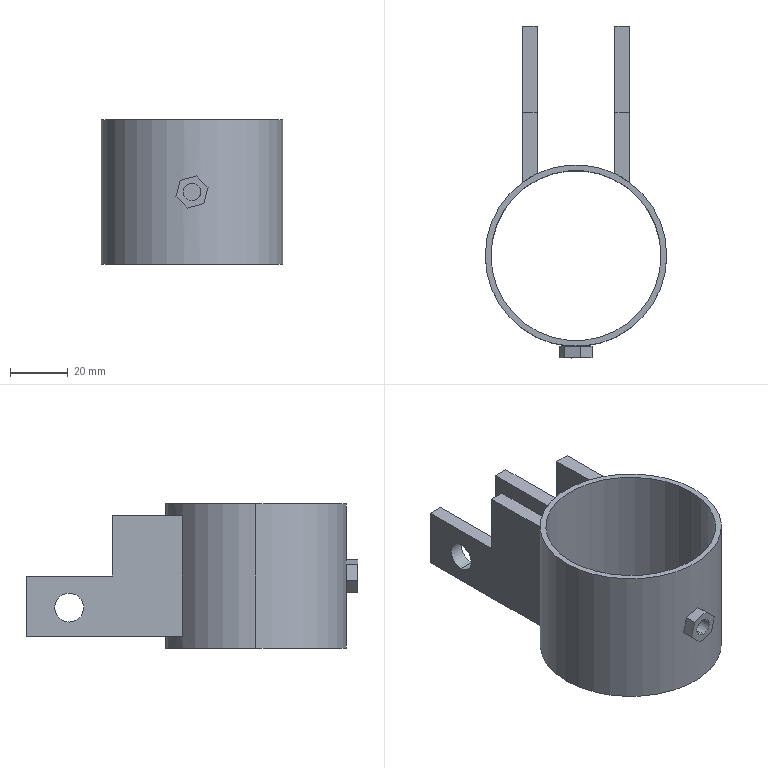Part | SolidWorks | features ICE 5, Extrusion 1 | 2 solids | 36 faces | box 63 x 115.25 x 50 mm | volume 34376 mm3 | plane 24 | cylinder 12 | commonest cylinder face diameters 6 x4 10 x4 59 x2 63 x2
STEP:
#1=CARTESIAN_POINT('',(0.,-31.5,22.));
#2=VERTEX_POINT('',#1);
#3=CARTESIAN_POINT('',(0.,-31.5,28.));
#4=VERTEX_POINT('',#3);
#5=CARTESIAN_POINT('',(0.,-31.5,22.));
#6=CARTESIAN_POINT('',(-0.1958,-31.5,22.));
#7=CARTESIAN_POINT('',(-0.3905,-31.498,22.019));
#8=CARTESIAN_POINT('',(-0.7776,-31.491,22.096));
#9=CARTESIAN_POINT('',(-0.967,-31.486,22.153));
#10=CARTESIAN_POINT('',(-1.328,-31.473,22.303));
#11=CARTESIAN_POINT('',(-1.502,-31.465,22.396));
#12=CARTESIAN_POINT('',(-1.83,-31.447,22.615));
#13=CARTESIAN_POINT('',(-1.981,-31.438,22.739));
#14=CARTESIAN_POINT('',(-2.258,-31.419,23.015));
#15=CARTESIAN_POINT('',(-2.385,-31.41,23.17));
#16=CARTESIAN_POINT('',(-2.603,-31.392,23.495));
#17=CARTESIAN_POINT('',(-2.695,-31.385,23.668));
#18=CARTESIAN_POINT('',(-2.846,-31.371,24.031));
#19=CARTESIAN_POINT('',(-2.904,-31.366,24.221));
#20=CARTESIAN_POINT('',(-2.98,-31.359,24.605));
#21=CARTESIAN_POINT('',(-3.,-31.357,24.8));
#22=CARTESIAN_POINT('',(-3.,-31.357,25.196));
#23=CARTESIAN_POINT('',(-2.981,-31.359,25.391));
#24=CARTESIAN_POINT('',(-2.905,-31.366,25.775));
#25=CARTESIAN_POINT('',(-2.847,-31.371,25.965));
#26=CARTESIAN_POINT('',(-2.697,-31.384,26.329));
#27=CARTESIAN_POINT('',(-2.605,-31.392,26.501));
#28=CARTESIAN_POINT('',(-2.388,-31.41,26.827));
#29=CARTESIAN_POINT('',(-2.261,-31.419,26.981));
#30=CARTESIAN_POINT('',(-1.985,-31.438,27.258));
#31=CARTESIAN_POINT('',(-1.834,-31.447,27.382));
#32=CARTESIAN_POINT('',(-1.506,-31.464,27.602));
#33=CARTESIAN_POINT('',(-1.332,-31.472,27.695));
#34=CARTESIAN_POINT('',(-0.7906,-31.492,27.92));
#35=CARTESIAN_POINT('',(-0.3966,-31.5,28.));
#36=CARTESIAN_POINT('',(0.,-31.5,28.));
#37=B_SPLINE_CURVE_WITH_KNOTS('',3,(#5,#6,#7,#8,#9,#10,#11,#12,#13,#14,#15,#16,#17,#18,#19,#20,#21,#22,#23,#24,#25,#26,#27,#28,#29,#30,#31,#32,#33,#34,#35,#36),.UNSPECIFIED.,.F.,.F.,(4,2,2,2,2,2,2,2,2,2,2,2,2,2,2,4),(0.009385,0.009971,0.01056,0.01114,0.01173,0.01232,0.0129,0.01349,0.01408,0.01466,0.01525,0.01584,0.01642,0.01701,0.01759,0.01877),.UNSPECIFIED.);
#38=EDGE_CURVE('',#2,#4,#37,.T.);
#39=ORIENTED_EDGE('',*,*,#38,.F.);
#40=CARTESIAN_POINT('',(0.,-29.5,22.));
#41=VERTEX_POINT('',#40);
#42=CARTESIAN_POINT('',(0.,-55.,22.));
#43=DIRECTION('',(0.,1.,0.));
#44=VECTOR('',#43,1000.);
#45=LINE('',#42,#44);
#46=EDGE_CURVE('',#2,#41,#45,.T.);
#47=ORIENTED_EDGE('',*,*,#46,.T.);
#48=CARTESIAN_POINT('',(0.,-29.5,28.));
#49=VERTEX_POINT('',#48);
#50=CARTESIAN_POINT('',(0.,-29.5,22.));
#51=CARTESIAN_POINT('',(-0.1958,-29.5,22.));
#52=CARTESIAN_POINT('',(-0.3905,-29.498,22.019));
#53=CARTESIAN_POINT('',(-0.7776,-29.49,22.096));
#54=CARTESIAN_POINT('',(-0.967,-29.485,22.153));
#55=CARTESIAN_POINT('',(-1.328,-29.471,22.303));
#56=CARTESIAN_POINT('',(-1.502,-29.462,22.396));
#57=CARTESIAN_POINT('',(-1.83,-29.444,22.615));
#58=CARTESIAN_POINT('',(-1.982,-29.434,22.739));
#59=CARTESIAN_POINT('',(-2.258,-29.414,23.015));
#60=CARTESIAN_POINT('',(-2.385,-29.404,23.17));
#61=CARTESIAN_POINT('',(-2.603,-29.385,23.495));
#62=CARTESIAN_POINT('',(-2.695,-29.377,23.668));
#63=CARTESIAN_POINT('',(-2.846,-29.363,24.031));
#64=CARTESIAN_POINT('',(-2.904,-29.357,24.221));
#65=CARTESIAN_POINT('',(-2.98,-29.349,24.605));
#66=CARTESIAN_POINT('',(-3.,-29.347,24.8));
#67=CARTESIAN_POINT('',(-3.,-29.347,25.196));
#68=CARTESIAN_POINT('',(-2.981,-29.349,25.391));
#69=CARTESIAN_POINT('',(-2.905,-29.357,25.775));
#70=CARTESIAN_POINT('',(-2.847,-29.362,25.965));
#71=CARTESIAN_POINT('',(-2.697,-29.377,26.329));
#72=CARTESIAN_POINT('',(-2.605,-29.385,26.501));
#73=CARTESIAN_POINT('',(-2.387,-29.403,26.827));
#74=CARTESIAN_POINT('',(-2.261,-29.414,26.981));
#75=CARTESIAN_POINT('',(-1.985,-29.433,27.258));
#76=CARTESIAN_POINT('',(-1.834,-29.443,27.382));
#77=CARTESIAN_POINT('',(-1.506,-29.462,27.602));
#78=CARTESIAN_POINT('',(-1.332,-29.47,27.695));
#79=CARTESIAN_POINT('',(-0.7907,-29.492,27.92));
#80=CARTESIAN_POINT('',(-0.3966,-29.5,28.));
#81=CARTESIAN_POINT('',(0.,-29.5,28.));
#82=B_SPLINE_CURVE_WITH_KNOTS('',3,(#50,#51,#52,#53,#54,#55,#56,#57,#58,#59,#60,#61,#62,#63,#64,#65,#66,#67,#68,#69,#70,#71,#72,#73,#74,#75,#76,#77,#78,#79,#80,#81),.UNSPECIFIED.,.F.,.F.,(4,2,2,2,2,2,2,2,2,2,2,2,2,2,2,4),(0.009385,0.009972,0.01056,0.01114,0.01173,0.01232,0.0129,0.01349,0.01408,0.01466,0.01525,0.01584,0.01642,0.01701,0.0176,0.01877),.UNSPECIFIED.);
#83=EDGE_CURVE('',#41,#49,#82,.T.);
#84=ORIENTED_EDGE('',*,*,#83,.T.);
#85=CARTESIAN_POINT('',(0.,-55.,28.));
#86=DIRECTION('',(0.,1.,0.));
#87=VECTOR('',#86,1000.);
#88=LINE('',#85,#87);
#89=EDGE_CURVE('',#4,#49,#88,.T.);
#90=ORIENTED_EDGE('',*,*,#89,.F.);
#91=EDGE_LOOP('',(#39,#47,#84,#90));
#92=FACE_OUTER_BOUND('',#91,.T.);
#93=CARTESIAN_POINT('',(0.,-55.,25.));
#94=DIRECTION('',(0.,1.,0.));
#95=DIRECTION('',(0.,0.,1.));
#96=AXIS2_PLACEMENT_3D('',#93,#94,#95);
#97=CYLINDRICAL_SURFACE('',#96,3.);
#98=ADVANCED_FACE('',(#92),#97,.F.);
#99=CARTESIAN_POINT('',(-13.5,64.75,9.));
#100=VERTEX_POINT('',#99);
#101=CARTESIAN_POINT('',(-13.5,64.75,19.));
#102=VERTEX_POINT('',#101);
#103=CARTESIAN_POINT('',(-13.5,64.75,14.));
#104=DIRECTION('',(-1.,0.,0.));
#105=DIRECTION('',(0.,0.,1.));
#106=AXIS2_PLACEMENT_3D('',#103,#104,#105);
#107=CIRCLE('',#106,5.);
#108=EDGE_CURVE('',#100,#102,#107,.T.);
#109=ORIENTED_EDGE('',*,*,#108,.F.);
#110=CARTESIAN_POINT('',(-18.5,64.75,9.));
#111=VERTEX_POINT('',#110);
#112=CARTESIAN_POINT('',(31.5,64.75,9.));
#113=DIRECTION('',(-1.,0.,0.));
#114=VECTOR('',#113,1000.);
#115=LINE('',#112,#114);
#116=EDGE_CURVE('',#100,#111,#115,.T.);
#117=ORIENTED_EDGE('',*,*,#116,.T.);
#118=CARTESIAN_POINT('',(-18.5,64.75,19.));
#119=VERTEX_POINT('',#118);
#120=CARTESIAN_POINT('',(-18.5,64.75,14.));
#121=DIRECTION('',(-1.,0.,0.));
#122=DIRECTION('',(0.,0.,1.));
#123=AXIS2_PLACEMENT_3D('',#120,#121,#122);
#124=CIRCLE('',#123,5.);
#125=EDGE_CURVE('',#111,#119,#124,.T.);
#126=ORIENTED_EDGE('',*,*,#125,.T.);
#127=CARTESIAN_POINT('',(31.5,64.75,19.));
#128=DIRECTION('',(-1.,0.,0.));
#129=VECTOR('',#128,1000.);
#130=LINE('',#127,#129);
#131=EDGE_CURVE('',#102,#119,#130,.T.);
#132=ORIENTED_EDGE('',*,*,#131,.F.);
#133=EDGE_LOOP('',(#109,#117,#126,#132));
#134=FACE_OUTER_BOUND('',#133,.T.);
#135=CARTESIAN_POINT('',(31.5,64.75,14.));
#136=DIRECTION('',(-1.,0.,0.));
#137=DIRECTION('',(0.,0.,1.));
#138=AXIS2_PLACEMENT_3D('',#135,#136,#137);
#139=CYLINDRICAL_SURFACE('',#138,5.);
#140=ADVANCED_FACE('',(#134),#139,.F.);
#141=CARTESIAN_POINT('',(18.5,64.75,9.));
#142=VERTEX_POINT('',#141);
#143=CARTESIAN_POINT('',(18.5,64.75,19.));
#144=VERTEX_POINT('',#143);
#145=CARTESIAN_POINT('',(18.5,64.75,14.));
#146=DIRECTION('',(-1.,0.,0.));
#147=DIRECTION('',(0.,0.,1.));
#148=AXIS2_PLACEMENT_3D('',#145,#146,#147);
#149=CIRCLE('',#148,5.);
#150=EDGE_CURVE('',#142,#144,#149,.T.);
#151=ORIENTED_EDGE('',*,*,#150,.F.);
#152=CARTESIAN_POINT('',(13.5,64.75,9.));
#153=VERTEX_POINT('',#152);
#154=CARTESIAN_POINT('',(31.5,64.75,9.));
#155=DIRECTION('',(-1.,0.,0.));
#156=VECTOR('',#155,1000.);
#157=LINE('',#154,#156);
#158=EDGE_CURVE('',#142,#153,#157,.T.);
#159=ORIENTED_EDGE('',*,*,#158,.T.);
#160=CARTESIAN_POINT('',(13.5,64.75,19.));
#161=VERTEX_POINT('',#160);
#162=CARTESIAN_POINT('',(13.5,64.75,14.));
#163=DIRECTION('',(1.,0.,0.));
#164=DIRECTION('',(0.,0.,-1.));
#165=AXIS2_PLACEMENT_3D('',#162,#163,#164);
#166=CIRCLE('',#165,5.);
#167=EDGE_CURVE('',#161,#153,#166,.T.);
#168=ORIENTED_EDGE('',*,*,#167,.F.);
#169=CARTESIAN_POINT('',(31.5,64.75,19.));
#170=DIRECTION('',(-1.,0.,0.));
#171=VECTOR('',#170,1000.);
#172=LINE('',#169,#171);
#173=EDGE_CURVE('',#144,#161,#172,.T.);
#174=ORIENTED_EDGE('',*,*,#173,.F.);
#175=EDGE_LOOP('',(#151,#159,#168,#174));
#176=FACE_OUTER_BOUND('',#175,.T.);
#177=CARTESIAN_POINT('',(31.5,64.75,14.));
#178=DIRECTION('',(-1.,0.,0.));
#179=DIRECTION('',(0.,0.,1.));
#180=AXIS2_PLACEMENT_3D('',#177,#178,#179);
#181=CYLINDRICAL_SURFACE('',#180,5.);
#182=ADVANCED_FACE('',(#176),#181,.F.);
#183=CARTESIAN_POINT('',(0.,-29.5,28.));
#184=CARTESIAN_POINT('',(0.1984,-29.5,28.));
#185=CARTESIAN_POINT('',(0.3934,-29.498,27.981));
#186=CARTESIAN_POINT('',(0.777,-29.49,27.904));
#187=CARTESIAN_POINT('',(0.9676,-29.485,27.846));
#188=CARTESIAN_POINT('',(1.331,-29.471,27.696));
#189=CARTESIAN_POINT('',(1.503,-29.462,27.604));
#190=CARTESIAN_POINT('',(1.829,-29.444,27.386));
#191=CARTESIAN_POINT('',(1.983,-29.434,27.259));
#192=CARTESIAN_POINT('',(2.26,-29.414,26.983));
#193=CARTESIAN_POINT('',(2.384,-29.404,26.832));
#194=CARTESIAN_POINT('',(2.603,-29.385,26.504));
#195=CARTESIAN_POINT('',(2.697,-29.377,26.329));
#196=CARTESIAN_POINT('',(2.846,-29.362,25.968));
#197=CARTESIAN_POINT('',(2.904,-29.357,25.779));
#198=CARTESIAN_POINT('',(2.981,-29.349,25.392));
#199=CARTESIAN_POINT('',(3.,-29.347,25.197));
#200=CARTESIAN_POINT('',(3.,-29.347,24.805));
#201=CARTESIAN_POINT('',(2.981,-29.349,24.606));
#202=CARTESIAN_POINT('',(2.904,-29.357,24.221));
#203=CARTESIAN_POINT('',(2.847,-29.362,24.034));
#204=CARTESIAN_POINT('',(2.697,-29.377,23.671));
#205=CARTESIAN_POINT('',(2.603,-29.385,23.496));
#206=CARTESIAN_POINT('',(2.386,-29.404,23.171));
#207=CARTESIAN_POINT('',(2.262,-29.414,23.019));
#208=CARTESIAN_POINT('',(1.982,-29.434,22.739));
#209=CARTESIAN_POINT('',(1.83,-29.444,22.615));
#210=CARTESIAN_POINT('',(1.505,-29.462,22.398));
#211=CARTESIAN_POINT('',(1.33,-29.471,22.304));
#212=CARTESIAN_POINT('',(0.9665,-29.485,22.153));
#213=CARTESIAN_POINT('',(0.7795,-29.49,22.096));
#214=CARTESIAN_POINT('',(0.3948,-29.498,22.02));
#215=CARTESIAN_POINT('',(0.1959,-29.5,22.));
#216=CARTESIAN_POINT('',(0.,-29.5,22.));
#217=B_SPLINE_CURVE_WITH_KNOTS('',3,(#183,#184,#185,#186,#187,#188,#189,#190,#191,#192,#193,#194,#195,#196,#197,#198,#199,#200,#201,#202,#203,#204,#205,#206,#207,#208,#209,#210,#211,#212,#213,#214,#215,#216),.UNSPECIFIED.,.F.,.F.,(4,2,2,2,2,2,2,2,2,2,2,2,2,2,2,2,4),(0.,0.0005866,0.001173,0.00176,0.002346,0.002933,0.00352,0.004106,0.004693,0.005279,0.005866,0.006452,0.007039,0.007626,0.008212,0.008799,0.009385),.UNSPECIFIED.);
#218=EDGE_CURVE('',#49,#41,#217,.T.);
#219=ORIENTED_EDGE('',*,*,#218,.F.);
#220=ORIENTED_EDGE('',*,*,#83,.F.);
#221=EDGE_LOOP('',(#219,#220));
#222=FACE_BOUND('',#221,.T.);
#223=CARTESIAN_POINT('',(-29.5,0.,50.));
#224=VERTEX_POINT('',#223);
#225=CARTESIAN_POINT('',(29.5,0.,50.));
#226=VERTEX_POINT('',#225);
#227=CARTESIAN_POINT('',(0.,0.,50.));
#228=DIRECTION('',(0.,0.,1.));
#229=DIRECTION('',(1.,0.,0.));
#230=AXIS2_PLACEMENT_3D('',#227,#228,#229);
#231=CIRCLE('',#230,29.5);
#232=EDGE_CURVE('',#224,#226,#231,.T.);
#233=ORIENTED_EDGE('',*,*,#232,.T.);
#234=CARTESIAN_POINT('',(29.5,0.,0.));
#235=VERTEX_POINT('',#234);
#236=CARTESIAN_POINT('',(29.5,0.,50.));
#237=DIRECTION('',(0.,0.,-1.));
#238=VECTOR('',#237,1000.);
#239=LINE('',#236,#238);
#240=EDGE_CURVE('',#226,#235,#239,.T.);
#241=ORIENTED_EDGE('',*,*,#240,.T.);
#242=CARTESIAN_POINT('',(-29.5,0.,0.));
#243=VERTEX_POINT('',#242);
#244=CARTESIAN_POINT('',(0.,0.,0.));
#245=DIRECTION('',(0.,0.,1.));
#246=DIRECTION('',(1.,0.,0.));
#247=AXIS2_PLACEMENT_3D('',#244,#245,#246);
#248=CIRCLE('',#247,29.5);
#249=EDGE_CURVE('',#243,#235,#248,.T.);
#250=ORIENTED_EDGE('',*,*,#249,.F.);
#251=CARTESIAN_POINT('',(-29.5,0.,50.));
#252=DIRECTION('',(0.,0.,-1.));
#253=VECTOR('',#252,1000.);
#254=LINE('',#251,#253);
#255=EDGE_CURVE('',#224,#243,#254,.T.);
#256=ORIENTED_EDGE('',*,*,#255,.F.);
#257=EDGE_LOOP('',(#233,#241,#250,#256));
#258=FACE_OUTER_BOUND('',#257,.T.);
#259=CARTESIAN_POINT('',(0.,0.,50.));
#260=DIRECTION('',(0.,0.,-1.));
#261=DIRECTION('',(-1.,0.,0.));
#262=AXIS2_PLACEMENT_3D('',#259,#260,#261);
#263=CYLINDRICAL_SURFACE('',#262,29.5);
#264=ADVANCED_FACE('',(#222,#258),#263,.F.);
#265=CARTESIAN_POINT('',(13.5,28.46,4.));
#266=VERTEX_POINT('',#265);
#267=CARTESIAN_POINT('',(13.5,28.46,46.));
#268=VERTEX_POINT('',#267);
#269=CARTESIAN_POINT('',(13.5,28.46,50.));
#270=DIRECTION('',(0.,0.,1.));
#271=VECTOR('',#270,1000.);
#272=LINE('',#269,#271);
#273=EDGE_CURVE('',#266,#268,#272,.T.);
#274=ORIENTED_EDGE('',*,*,#273,.F.);
#275=CARTESIAN_POINT('',(18.5,25.495,4.));
#276=VERTEX_POINT('',#275);
#277=CARTESIAN_POINT('',(0.,0.,4.));
#278=DIRECTION('',(0.,0.,1.));
#279=DIRECTION('',(-1.,0.,0.));
#280=AXIS2_PLACEMENT_3D('',#277,#278,#279);
#281=CIRCLE('',#280,31.5);
#282=EDGE_CURVE('',#276,#266,#281,.T.);
#283=ORIENTED_EDGE('',*,*,#282,.F.);
#284=CARTESIAN_POINT('',(18.5,25.495,46.));
#285=VERTEX_POINT('',#284);
#286=CARTESIAN_POINT('',(18.5,25.495,50.));
#287=DIRECTION('',(0.,0.,-1.));
#288=VECTOR('',#287,1000.);
#289=LINE('',#286,#288);
#290=EDGE_CURVE('',#285,#276,#289,.T.);
#291=ORIENTED_EDGE('',*,*,#290,.F.);
#292=CARTESIAN_POINT('',(0.,0.,46.));
#293=DIRECTION('',(0.,0.,-1.));
#294=DIRECTION('',(1.,0.,0.));
#295=AXIS2_PLACEMENT_3D('',#292,#293,#294);
#296=CIRCLE('',#295,31.5);
#297=EDGE_CURVE('',#268,#285,#296,.T.);
#298=ORIENTED_EDGE('',*,*,#297,.F.);
#299=EDGE_LOOP('',(#274,#283,#291,#298));
#300=FACE_BOUND('',#299,.T.);
#301=CARTESIAN_POINT('',(-18.5,25.495,4.));
#302=VERTEX_POINT('',#301);
#303=CARTESIAN_POINT('',(-18.5,25.495,46.));
#304=VERTEX_POINT('',#303);
#305=CARTESIAN_POINT('',(-18.5,25.495,50.));
#306=DIRECTION('',(0.,0.,1.));
#307=VECTOR('',#306,1000.);
#308=LINE('',#305,#307);
#309=EDGE_CURVE('',#302,#304,#308,.T.);
#310=ORIENTED_EDGE('',*,*,#309,.F.);
#311=CARTESIAN_POINT('',(-13.5,28.46,4.));
#312=VERTEX_POINT('',#311);
#313=CARTESIAN_POINT('',(0.,0.,4.));
#314=DIRECTION('',(0.,0.,1.));
#315=DIRECTION('',(-1.,0.,0.));
#316=AXIS2_PLACEMENT_3D('',#313,#314,#315);
#317=CIRCLE('',#316,31.5);
#318=EDGE_CURVE('',#312,#302,#317,.T.);
#319=ORIENTED_EDGE('',*,*,#318,.F.);
#320=CARTESIAN_POINT('',(-13.5,28.46,46.));
#321=VERTEX_POINT('',#320);
#322=CARTESIAN_POINT('',(-13.5,28.46,50.));
#323=DIRECTION('',(0.,0.,-1.));
#324=VECTOR('',#323,1000.);
#325=LINE('',#322,#324);
#326=EDGE_CURVE('',#321,#312,#325,.T.);
#327=ORIENTED_EDGE('',*,*,#326,.F.);
#328=CARTESIAN_POINT('',(0.,0.,46.));
#329=DIRECTION('',(0.,0.,-1.));
#330=DIRECTION('',(1.,0.,0.));
#331=AXIS2_PLACEMENT_3D('',#328,#329,#330);
#332=CIRCLE('',#331,31.5);
#333=EDGE_CURVE('',#304,#321,#332,.T.);
#334=ORIENTED_EDGE('',*,*,#333,.F.);
#335=EDGE_LOOP('',(#310,#319,#327,#334));
#336=FACE_BOUND('',#335,.T.);
#337=CARTESIAN_POINT('',(31.5,0.,50.));
#338=VERTEX_POINT('',#337);
#339=CARTESIAN_POINT('',(-31.5,0.,50.));
#340=VERTEX_POINT('',#339);
#341=CARTESIAN_POINT('',(0.,0.,50.));
#342=DIRECTION('',(0.,0.,1.));
#343=DIRECTION('',(1.,0.,0.));
#344=AXIS2_PLACEMENT_3D('',#341,#342,#343);
#345=CIRCLE('',#344,31.5);
#346=EDGE_CURVE('',#338,#340,#345,.T.);
#347=ORIENTED_EDGE('',*,*,#346,.F.);
#348=CARTESIAN_POINT('',(31.5,0.,0.));
#349=VERTEX_POINT('',#348);
#350=CARTESIAN_POINT('',(31.5,0.,50.));
#351=DIRECTION('',(0.,0.,-1.));
#352=VECTOR('',#351,1000.);
#353=LINE('',#350,#352);
#354=EDGE_CURVE('',#338,#349,#353,.T.);
#355=ORIENTED_EDGE('',*,*,#354,.T.);
#356=CARTESIAN_POINT('',(-31.5,0.,0.));
#357=VERTEX_POINT('',#356);
#358=CARTESIAN_POINT('',(0.,0.,0.));
#359=DIRECTION('',(0.,0.,1.));
#360=DIRECTION('',(1.,0.,0.));
#361=AXIS2_PLACEMENT_3D('',#358,#359,#360);
#362=CIRCLE('',#361,31.5);
#363=EDGE_CURVE('',#349,#357,#362,.T.);
#364=ORIENTED_EDGE('',*,*,#363,.T.);
#365=CARTESIAN_POINT('',(-31.5,0.,50.));
#366=DIRECTION('',(0.,0.,-1.));
#367=VECTOR('',#366,1000.);
#368=LINE('',#365,#367);
#369=EDGE_CURVE('',#340,#357,#368,.T.);
#370=ORIENTED_EDGE('',*,*,#369,.F.);
#371=EDGE_LOOP('',(#347,#355,#364,#370));
#372=FACE_OUTER_BOUND('',#371,.T.);
#373=CARTESIAN_POINT('',(0.,0.,50.));
#374=DIRECTION('',(0.,0.,-1.));
#375=DIRECTION('',(-1.,0.,0.));
#376=AXIS2_PLACEMENT_3D('',#373,#374,#375);
#377=CYLINDRICAL_SURFACE('',#376,31.5);
#378=ADVANCED_FACE('',(#300,#336,#372),#377,.T.);
#379=ORIENTED_EDGE('',*,*,#354,.F.);
#380=CARTESIAN_POINT('',(0.,0.,50.));
#381=DIRECTION('',(0.,0.,1.));
#382=DIRECTION('',(1.,0.,0.));
#383=AXIS2_PLACEMENT_3D('',#380,#381,#382);
#384=CIRCLE('',#383,31.5);
#385=EDGE_CURVE('',#340,#338,#384,.T.);
#386=ORIENTED_EDGE('',*,*,#385,.F.);
#387=ORIENTED_EDGE('',*,*,#369,.T.);
#388=CARTESIAN_POINT('',(0.,0.,0.));
#389=DIRECTION('',(0.,0.,1.));
#390=DIRECTION('',(1.,0.,0.));
#391=AXIS2_PLACEMENT_3D('',#388,#389,#390);
#392=CIRCLE('',#391,31.5);
#393=EDGE_CURVE('',#357,#349,#392,.T.);
#394=ORIENTED_EDGE('',*,*,#393,.T.);
#395=EDGE_LOOP('',(#379,#386,#387,#394));
#396=FACE_OUTER_BOUND('',#395,.T.);
#397=CARTESIAN_POINT('',(0.,-31.5,28.));
#398=CARTESIAN_POINT('',(0.1983,-31.5,28.));
#399=CARTESIAN_POINT('',(0.3933,-31.498,27.981));
#400=CARTESIAN_POINT('',(0.7769,-31.491,27.904));
#401=CARTESIAN_POINT('',(0.9675,-31.486,27.846));
#402=CARTESIAN_POINT('',(1.331,-31.472,27.696));
#403=CARTESIAN_POINT('',(1.503,-31.465,27.604));
#404=CARTESIAN_POINT('',(1.829,-31.447,27.386));
#405=CARTESIAN_POINT('',(1.983,-31.438,27.259));
#406=CARTESIAN_POINT('',(2.26,-31.419,26.983));
#407=CARTESIAN_POINT('',(2.384,-31.41,26.832));
#408=CARTESIAN_POINT('',(2.603,-31.392,26.504));
#409=CARTESIAN_POINT('',(2.697,-31.384,26.329));
#410=CARTESIAN_POINT('',(2.846,-31.371,25.968));
#411=CARTESIAN_POINT('',(2.904,-31.366,25.779));
#412=CARTESIAN_POINT('',(2.981,-31.359,25.392));
#413=CARTESIAN_POINT('',(3.,-31.357,25.197));
#414=CARTESIAN_POINT('',(3.,-31.357,24.805));
#415=CARTESIAN_POINT('',(2.981,-31.359,24.606));
#416=CARTESIAN_POINT('',(2.904,-31.366,24.222));
#417=CARTESIAN_POINT('',(2.847,-31.371,24.034));
#418=CARTESIAN_POINT('',(2.697,-31.384,23.671));
#419=CARTESIAN_POINT('',(2.603,-31.392,23.496));
#420=CARTESIAN_POINT('',(2.386,-31.41,23.171));
#421=CARTESIAN_POINT('',(2.262,-31.419,23.019));
#422=CARTESIAN_POINT('',(1.982,-31.438,22.739));
#423=CARTESIAN_POINT('',(1.83,-31.447,22.615));
#424=CARTESIAN_POINT('',(1.505,-31.464,22.398));
#425=CARTESIAN_POINT('',(1.33,-31.472,22.304));
#426=CARTESIAN_POINT('',(0.9665,-31.486,22.153));
#427=CARTESIAN_POINT('',(0.7794,-31.491,22.096));
#428=CARTESIAN_POINT('',(0.3948,-31.498,22.02));
#429=CARTESIAN_POINT('',(0.1959,-31.5,22.));
#430=CARTESIAN_POINT('',(0.,-31.5,22.));
#431=B_SPLINE_CURVE_WITH_KNOTS('',3,(#397,#398,#399,#400,#401,#402,#403,#404,#405,#406,#407,#408,#409,#410,#411,#412,#413,#414,#415,#416,#417,#418,#419,#420,#421,#422,#423,#424,#425,#426,#427,#428,#429,#430),.UNSPECIFIED.,.F.,.F.,(4,2,2,2,2,2,2,2,2,2,2,2,2,2,2,2,4),(0.,0.0005865,0.001173,0.00176,0.002346,0.002933,0.003519,0.004106,0.004692,0.005279,0.005865,0.006452,0.007039,0.007625,0.008212,0.008798,0.009385),.UNSPECIFIED.);
#432=EDGE_CURVE('',#4,#2,#431,.T.);
#433=ORIENTED_EDGE('',*,*,#432,.T.);
#434=ORIENTED_EDGE('',*,*,#38,.T.);
#435=EDGE_LOOP('',(#433,#434));
#436=FACE_BOUND('',#435,.T.);
#437=CARTESIAN_POINT('',(0.,0.,50.));
#438=DIRECTION('',(0.,0.,-1.));
#439=DIRECTION('',(-1.,0.,0.));
#440=AXIS2_PLACEMENT_3D('',#437,#438,#439);
#441=CYLINDRICAL_SURFACE('',#440,31.5);
#442=ADVANCED_FACE('',(#396,#436),#441,.T.);
#443=ORIENTED_EDGE('',*,*,#385,.T.);
#444=ORIENTED_EDGE('',*,*,#346,.T.);
#445=EDGE_LOOP('',(#443,#444));
#446=FACE_OUTER_BOUND('',#445,.T.);
#447=ORIENTED_EDGE('',*,*,#232,.F.);
#448=CARTESIAN_POINT('',(0.,0.,50.));
#449=DIRECTION('',(0.,0.,1.));
#450=DIRECTION('',(1.,0.,0.));
#451=AXIS2_PLACEMENT_3D('',#448,#449,#450);
#452=CIRCLE('',#451,29.5);
#453=EDGE_CURVE('',#226,#224,#452,.T.);
#454=ORIENTED_EDGE('',*,*,#453,.F.);
#455=EDGE_LOOP('',(#447,#454));
#456=FACE_BOUND('',#455,.T.);
#457=CARTESIAN_POINT('',(0.,0.,50.));
#458=DIRECTION('',(0.,0.,1.));
#459=DIRECTION('',(1.,0.,0.));
#460=AXIS2_PLACEMENT_3D('',#457,#458,#459);
#461=PLANE('',#460);
#462=ADVANCED_FACE('',(#446,#456),#461,.T.);
#463=ORIENTED_EDGE('',*,*,#393,.F.);
#464=ORIENTED_EDGE('',*,*,#363,.F.);
#465=EDGE_LOOP('',(#463,#464));
#466=FACE_OUTER_BOUND('',#465,.T.);
#467=ORIENTED_EDGE('',*,*,#249,.T.);
#468=CARTESIAN_POINT('',(0.,0.,0.));
#469=DIRECTION('',(0.,0.,1.));
#470=DIRECTION('',(1.,0.,0.));
#471=AXIS2_PLACEMENT_3D('',#468,#469,#470);
#472=CIRCLE('',#471,29.5);
#473=EDGE_CURVE('',#235,#243,#472,.T.);
#474=ORIENTED_EDGE('',*,*,#473,.T.);
#475=EDGE_LOOP('',(#467,#474));
#476=FACE_BOUND('',#475,.T.);
#477=CARTESIAN_POINT('',(0.,0.,0.));
#478=DIRECTION('',(0.,0.,1.));
#479=DIRECTION('',(1.,0.,0.));
#480=AXIS2_PLACEMENT_3D('',#477,#478,#479);
#481=PLANE('',#480);
#482=ADVANCED_FACE('',(#466,#476),#481,.F.);
#483=ORIENTED_EDGE('',*,*,#240,.F.);
#484=ORIENTED_EDGE('',*,*,#453,.T.);
#485=ORIENTED_EDGE('',*,*,#255,.T.);
#486=ORIENTED_EDGE('',*,*,#473,.F.);
#487=EDGE_LOOP('',(#483,#484,#485,#486));
#488=FACE_OUTER_BOUND('',#487,.T.);
#489=CARTESIAN_POINT('',(0.,0.,50.));
#490=DIRECTION('',(0.,0.,-1.));
#491=DIRECTION('',(-1.,0.,0.));
#492=AXIS2_PLACEMENT_3D('',#489,#490,#491);
#493=CYLINDRICAL_SURFACE('',#492,29.5);
#494=ADVANCED_FACE('',(#488),#493,.F.);
#495=CARTESIAN_POINT('',(-18.5,64.75,14.));
#496=DIRECTION('',(-1.,0.,0.));
#497=DIRECTION('',(0.,0.,1.));
#498=AXIS2_PLACEMENT_3D('',#495,#496,#497);
#499=CIRCLE('',#498,5.);
#500=EDGE_CURVE('',#119,#111,#499,.T.);
#501=ORIENTED_EDGE('',*,*,#500,.F.);
#502=ORIENTED_EDGE('',*,*,#125,.F.);
#503=EDGE_LOOP('',(#501,#502));
#504=FACE_BOUND('',#503,.T.);
#505=CARTESIAN_POINT('',(-18.5,49.75,46.));
#506=VERTEX_POINT('',#505);
#507=CARTESIAN_POINT('',(-18.5,79.75,46.));
#508=DIRECTION('',(0.,-1.,0.));
#509=VECTOR('',#508,1000.);
#510=LINE('',#507,#509);
#511=EDGE_CURVE('',#506,#304,#510,.T.);
#512=ORIENTED_EDGE('',*,*,#511,.F.);
#513=CARTESIAN_POINT('',(-18.5,49.75,25.));
#514=VERTEX_POINT('',#513);
#515=CARTESIAN_POINT('',(-18.5,49.75,25.));
#516=DIRECTION('',(0.,0.,1.));
#517=VECTOR('',#516,1000.);
#518=LINE('',#515,#517);
#519=EDGE_CURVE('',#514,#506,#518,.T.);
#520=ORIENTED_EDGE('',*,*,#519,.F.);
#521=CARTESIAN_POINT('',(-18.5,79.75,25.));
#522=VERTEX_POINT('',#521);
#523=CARTESIAN_POINT('',(-18.5,79.75,25.));
#524=DIRECTION('',(0.,-1.,0.));
#525=VECTOR('',#524,1000.);
#526=LINE('',#523,#525);
#527=EDGE_CURVE('',#522,#514,#526,.T.);
#528=ORIENTED_EDGE('',*,*,#527,.F.);
#529=CARTESIAN_POINT('',(-18.5,79.75,4.));
#530=VERTEX_POINT('',#529);
#531=CARTESIAN_POINT('',(-18.5,79.75,46.));
#532=DIRECTION('',(0.,0.,1.));
#533=VECTOR('',#532,1000.);
#534=LINE('',#531,#533);
#535=EDGE_CURVE('',#530,#522,#534,.T.);
#536=ORIENTED_EDGE('',*,*,#535,.F.);
#537=CARTESIAN_POINT('',(-18.5,79.75,4.));
#538=DIRECTION('',(0.,-1.,0.));
#539=VECTOR('',#538,1000.);
#540=LINE('',#537,#539);
#541=EDGE_CURVE('',#530,#302,#540,.T.);
#542=ORIENTED_EDGE('',*,*,#541,.T.);
#543=ORIENTED_EDGE('',*,*,#309,.T.);
#544=EDGE_LOOP('',(#512,#520,#528,#536,#542,#543));
#545=FACE_OUTER_BOUND('',#544,.T.);
#546=CARTESIAN_POINT('',(-18.5,79.75,46.));
#547=DIRECTION('',(1.,0.,0.));
#548=DIRECTION('',(0.,0.,-1.));
#549=AXIS2_PLACEMENT_3D('',#546,#547,#548);
#550=PLANE('',#549);
#551=ADVANCED_FACE('',(#504,#545),#550,.F.);
#552=CARTESIAN_POINT('',(-13.5,49.75,46.));
#553=VERTEX_POINT('',#552);
#554=CARTESIAN_POINT('',(-13.5,79.75,46.));
#555=DIRECTION('',(0.,-1.,0.));
#556=VECTOR('',#555,1000.);
#557=LINE('',#554,#556);
#558=EDGE_CURVE('',#553,#321,#557,.T.);
#559=ORIENTED_EDGE('',*,*,#558,.F.);
#560=CARTESIAN_POINT('',(31.5,49.75,46.));
#561=DIRECTION('',(-1.,0.,0.));
#562=VECTOR('',#561,1000.);
#563=LINE('',#560,#562);
#564=EDGE_CURVE('',#553,#506,#563,.T.);
#565=ORIENTED_EDGE('',*,*,#564,.T.);
#566=ORIENTED_EDGE('',*,*,#511,.T.);
#567=ORIENTED_EDGE('',*,*,#333,.T.);
#568=EDGE_LOOP('',(#559,#565,#566,#567));
#569=FACE_OUTER_BOUND('',#568,.T.);
#570=CARTESIAN_POINT('',(-13.5,79.75,46.));
#571=DIRECTION('',(0.,0.,-1.));
#572=DIRECTION('',(-1.,0.,0.));
#573=AXIS2_PLACEMENT_3D('',#570,#571,#572);
#574=PLANE('',#573);
#575=ADVANCED_FACE('',(#569),#574,.F.);
#576=CARTESIAN_POINT('',(-13.5,64.75,14.));
#577=DIRECTION('',(-1.,0.,0.));
#578=DIRECTION('',(0.,0.,1.));
#579=AXIS2_PLACEMENT_3D('',#576,#577,#578);
#580=CIRCLE('',#579,5.);
#581=EDGE_CURVE('',#102,#100,#580,.T.);
#582=ORIENTED_EDGE('',*,*,#581,.T.);
#583=ORIENTED_EDGE('',*,*,#108,.T.);
#584=EDGE_LOOP('',(#582,#583));
#585=FACE_BOUND('',#584,.T.);
#586=CARTESIAN_POINT('',(-13.5,79.75,25.));
#587=VERTEX_POINT('',#586);
#588=CARTESIAN_POINT('',(-13.5,49.75,25.));
#589=VERTEX_POINT('',#588);
#590=CARTESIAN_POINT('',(-13.5,79.75,25.));
#591=DIRECTION('',(0.,-1.,0.));
#592=VECTOR('',#591,1000.);
#593=LINE('',#590,#592);
#594=EDGE_CURVE('',#587,#589,#593,.T.);
#595=ORIENTED_EDGE('',*,*,#594,.T.);
#596=CARTESIAN_POINT('',(-13.5,49.75,46.));
#597=DIRECTION('',(0.,0.,1.));
#598=VECTOR('',#597,1000.);
#599=LINE('',#596,#598);
#600=EDGE_CURVE('',#589,#553,#599,.T.);
#601=ORIENTED_EDGE('',*,*,#600,.T.);
#602=ORIENTED_EDGE('',*,*,#558,.T.);
#603=ORIENTED_EDGE('',*,*,#326,.T.);
#604=CARTESIAN_POINT('',(-13.5,79.75,4.));
#605=VERTEX_POINT('',#604);
#606=CARTESIAN_POINT('',(-13.5,79.75,4.));
#607=DIRECTION('',(0.,-1.,0.));
#608=VECTOR('',#607,1000.);
#609=LINE('',#606,#608);
#610=EDGE_CURVE('',#605,#312,#609,.T.);
#611=ORIENTED_EDGE('',*,*,#610,.F.);
#612=CARTESIAN_POINT('',(-13.5,79.75,46.));
#613=DIRECTION('',(0.,0.,-1.));
#614=VECTOR('',#613,1000.);
#615=LINE('',#612,#614);
#616=EDGE_CURVE('',#587,#605,#615,.T.);
#617=ORIENTED_EDGE('',*,*,#616,.F.);
#618=EDGE_LOOP('',(#595,#601,#602,#603,#611,#617));
#619=FACE_OUTER_BOUND('',#618,.T.);
#620=CARTESIAN_POINT('',(-13.5,79.75,46.));
#621=DIRECTION('',(-1.,0.,0.));
#622=DIRECTION('',(0.,0.,1.));
#623=AXIS2_PLACEMENT_3D('',#620,#621,#622);
#624=PLANE('',#623);
#625=ADVANCED_FACE('',(#585,#619),#624,.F.);
#626=ORIENTED_EDGE('',*,*,#610,.T.);
#627=ORIENTED_EDGE('',*,*,#318,.T.);
#628=ORIENTED_EDGE('',*,*,#541,.F.);
#629=CARTESIAN_POINT('',(-13.5,79.75,4.));
#630=DIRECTION('',(-1.,0.,0.));
#631=VECTOR('',#630,1000.);
#632=LINE('',#629,#631);
#633=EDGE_CURVE('',#605,#530,#632,.T.);
#634=ORIENTED_EDGE('',*,*,#633,.F.);
#635=EDGE_LOOP('',(#626,#627,#628,#634));
#636=FACE_OUTER_BOUND('',#635,.T.);
#637=CARTESIAN_POINT('',(-13.5,79.75,4.));
#638=DIRECTION('',(0.,0.,1.));
#639=DIRECTION('',(1.,0.,0.));
#640=AXIS2_PLACEMENT_3D('',#637,#638,#639);
#641=PLANE('',#640);
#642=ADVANCED_FACE('',(#636),#641,.F.);
#643=CARTESIAN_POINT('',(31.5,79.75,25.));
#644=DIRECTION('',(-1.,0.,0.));
#645=VECTOR('',#644,1000.);
#646=LINE('',#643,#645);
#647=EDGE_CURVE('',#587,#522,#646,.T.);
#648=ORIENTED_EDGE('',*,*,#647,.F.);
#649=ORIENTED_EDGE('',*,*,#616,.T.);
#650=ORIENTED_EDGE('',*,*,#633,.T.);
#651=ORIENTED_EDGE('',*,*,#535,.T.);
#652=EDGE_LOOP('',(#648,#649,#650,#651));
#653=FACE_OUTER_BOUND('',#652,.T.);
#654=CARTESIAN_POINT('',(0.,79.75,0.));
#655=DIRECTION('',(0.,1.,0.));
#656=DIRECTION('',(0.,0.,1.));
#657=AXIS2_PLACEMENT_3D('',#654,#655,#656);
#658=PLANE('',#657);
#659=ADVANCED_FACE('',(#653),#658,.T.);
#660=ORIENTED_EDGE('',*,*,#167,.T.);
#661=CARTESIAN_POINT('',(13.5,64.75,14.));
#662=DIRECTION('',(1.,0.,0.));
#663=DIRECTION('',(0.,0.,-1.));
#664=AXIS2_PLACEMENT_3D('',#661,#662,#663);
#665=CIRCLE('',#664,5.);
#666=EDGE_CURVE('',#153,#161,#665,.T.);
#667=ORIENTED_EDGE('',*,*,#666,.T.);
#668=EDGE_LOOP('',(#660,#667));
#669=FACE_BOUND('',#668,.T.);
#670=CARTESIAN_POINT('',(13.5,49.75,46.));
#671=VERTEX_POINT('',#670);
#672=CARTESIAN_POINT('',(13.5,79.75,46.));
#673=DIRECTION('',(0.,-1.,0.));
#674=VECTOR('',#673,1000.);
#675=LINE('',#672,#674);
#676=EDGE_CURVE('',#671,#268,#675,.T.);
#677=ORIENTED_EDGE('',*,*,#676,.F.);
#678=CARTESIAN_POINT('',(13.5,49.75,25.));
#679=VERTEX_POINT('',#678);
#680=CARTESIAN_POINT('',(13.5,49.75,46.));
#681=DIRECTION('',(0.,0.,-1.));
#682=VECTOR('',#681,1000.);
#683=LINE('',#680,#682);
#684=EDGE_CURVE('',#671,#679,#683,.T.);
#685=ORIENTED_EDGE('',*,*,#684,.T.);
#686=CARTESIAN_POINT('',(13.5,79.75,25.));
#687=VERTEX_POINT('',#686);
#688=CARTESIAN_POINT('',(13.5,79.75,25.));
#689=DIRECTION('',(0.,1.,0.));
#690=VECTOR('',#689,1000.);
#691=LINE('',#688,#690);
#692=EDGE_CURVE('',#679,#687,#691,.T.);
#693=ORIENTED_EDGE('',*,*,#692,.T.);
#694=CARTESIAN_POINT('',(13.5,79.75,4.));
#695=VERTEX_POINT('',#694);
#696=CARTESIAN_POINT('',(13.5,79.75,46.));
#697=DIRECTION('',(0.,0.,1.));
#698=VECTOR('',#697,1000.);
#699=LINE('',#696,#698);
#700=EDGE_CURVE('',#695,#687,#699,.T.);
#701=ORIENTED_EDGE('',*,*,#700,.F.);
#702=CARTESIAN_POINT('',(13.5,79.75,4.));
#703=DIRECTION('',(0.,-1.,0.));
#704=VECTOR('',#703,1000.);
#705=LINE('',#702,#704);
#706=EDGE_CURVE('',#695,#266,#705,.T.);
#707=ORIENTED_EDGE('',*,*,#706,.T.);
#708=ORIENTED_EDGE('',*,*,#273,.T.);
#709=EDGE_LOOP('',(#677,#685,#693,#701,#707,#708));
#710=FACE_OUTER_BOUND('',#709,.T.);
#711=CARTESIAN_POINT('',(13.5,79.75,46.));
#712=DIRECTION('',(1.,0.,0.));
#713=DIRECTION('',(0.,0.,-1.));
#714=AXIS2_PLACEMENT_3D('',#711,#712,#713);
#715=PLANE('',#714);
#716=ADVANCED_FACE('',(#669,#710),#715,.F.);
#717=CARTESIAN_POINT('',(18.5,49.75,46.));
#718=VERTEX_POINT('',#717);
#719=CARTESIAN_POINT('',(18.5,79.75,46.));
#720=DIRECTION('',(0.,-1.,0.));
#721=VECTOR('',#720,1000.);
#722=LINE('',#719,#721);
#723=EDGE_CURVE('',#718,#285,#722,.T.);
#724=ORIENTED_EDGE('',*,*,#723,.F.);
#725=CARTESIAN_POINT('',(31.5,49.75,46.));
#726=DIRECTION('',(-1.,0.,0.));
#727=VECTOR('',#726,1000.);
#728=LINE('',#725,#727);
#729=EDGE_CURVE('',#718,#671,#728,.T.);
#730=ORIENTED_EDGE('',*,*,#729,.T.);
#731=ORIENTED_EDGE('',*,*,#676,.T.);
#732=ORIENTED_EDGE('',*,*,#297,.T.);
#733=EDGE_LOOP('',(#724,#730,#731,#732));
#734=FACE_OUTER_BOUND('',#733,.T.);
#735=CARTESIAN_POINT('',(13.5,79.75,46.));
#736=DIRECTION('',(0.,0.,-1.));
#737=DIRECTION('',(-1.,0.,0.));
#738=AXIS2_PLACEMENT_3D('',#735,#736,#737);
#739=PLANE('',#738);
#740=ADVANCED_FACE('',(#734),#739,.F.);
#741=CARTESIAN_POINT('',(18.5,64.75,14.));
#742=DIRECTION('',(-1.,0.,0.));
#743=DIRECTION('',(0.,0.,1.));
#744=AXIS2_PLACEMENT_3D('',#741,#742,#743);
#745=CIRCLE('',#744,5.);
#746=EDGE_CURVE('',#144,#142,#745,.T.);
#747=ORIENTED_EDGE('',*,*,#746,.T.);
#748=ORIENTED_EDGE('',*,*,#150,.T.);
#749=EDGE_LOOP('',(#747,#748));
#750=FACE_BOUND('',#749,.T.);
#751=CARTESIAN_POINT('',(18.5,79.75,25.));
#752=VERTEX_POINT('',#751);
#753=CARTESIAN_POINT('',(18.5,49.75,25.));
#754=VERTEX_POINT('',#753);
#755=CARTESIAN_POINT('',(18.5,79.75,25.));
#756=DIRECTION('',(0.,-1.,0.));
#757=VECTOR('',#756,1000.);
#758=LINE('',#755,#757);
#759=EDGE_CURVE('',#752,#754,#758,.T.);
#760=ORIENTED_EDGE('',*,*,#759,.T.);
#761=CARTESIAN_POINT('',(18.5,49.75,46.));
#762=DIRECTION('',(0.,0.,1.));
#763=VECTOR('',#762,1000.);
#764=LINE('',#761,#763);
#765=EDGE_CURVE('',#754,#718,#764,.T.);
#766=ORIENTED_EDGE('',*,*,#765,.T.);
#767=ORIENTED_EDGE('',*,*,#723,.T.);
#768=ORIENTED_EDGE('',*,*,#290,.T.);
#769=CARTESIAN_POINT('',(18.5,79.75,4.));
#770=VERTEX_POINT('',#769);
#771=CARTESIAN_POINT('',(18.5,79.75,4.));
#772=DIRECTION('',(0.,-1.,0.));
#773=VECTOR('',#772,1000.);
#774=LINE('',#771,#773);
#775=EDGE_CURVE('',#770,#276,#774,.T.);
#776=ORIENTED_EDGE('',*,*,#775,.F.);
#777=CARTESIAN_POINT('',(18.5,79.75,46.));
#778=DIRECTION('',(0.,0.,-1.));
#779=VECTOR('',#778,1000.);
#780=LINE('',#777,#779);
#781=EDGE_CURVE('',#752,#770,#780,.T.);
#782=ORIENTED_EDGE('',*,*,#781,.F.);
#783=EDGE_LOOP('',(#760,#766,#767,#768,#776,#782));
#784=FACE_OUTER_BOUND('',#783,.T.);
#785=CARTESIAN_POINT('',(18.5,79.75,46.));
#786=DIRECTION('',(-1.,0.,0.));
#787=DIRECTION('',(0.,0.,1.));
#788=AXIS2_PLACEMENT_3D('',#785,#786,#787);
#789=PLANE('',#788);
#790=ADVANCED_FACE('',(#750,#784),#789,.F.);
#791=ORIENTED_EDGE('',*,*,#775,.T.);
#792=ORIENTED_EDGE('',*,*,#282,.T.);
#793=ORIENTED_EDGE('',*,*,#706,.F.);
#794=CARTESIAN_POINT('',(13.5,79.75,4.));
#795=DIRECTION('',(-1.,0.,0.));
#796=VECTOR('',#795,1000.);
#797=LINE('',#794,#796);
#798=EDGE_CURVE('',#770,#695,#797,.T.);
#799=ORIENTED_EDGE('',*,*,#798,.F.);
#800=EDGE_LOOP('',(#791,#792,#793,#799));
#801=FACE_OUTER_BOUND('',#800,.T.);
#802=CARTESIAN_POINT('',(13.5,79.75,4.));
#803=DIRECTION('',(0.,0.,1.));
#804=DIRECTION('',(1.,0.,0.));
#805=AXIS2_PLACEMENT_3D('',#802,#803,#804);
#806=PLANE('',#805);
#807=ADVANCED_FACE('',(#801),#806,.F.);
#808=ORIENTED_EDGE('',*,*,#700,.T.);
#809=CARTESIAN_POINT('',(0.,79.75,25.));
#810=DIRECTION('',(1.,0.,0.));
#811=VECTOR('',#810,1000.);
#812=LINE('',#809,#811);
#813=EDGE_CURVE('',#687,#752,#812,.T.);
#814=ORIENTED_EDGE('',*,*,#813,.T.);
#815=ORIENTED_EDGE('',*,*,#781,.T.);
#816=ORIENTED_EDGE('',*,*,#798,.T.);
#817=EDGE_LOOP('',(#808,#814,#815,#816));
#818=FACE_OUTER_BOUND('',#817,.T.);
#819=CARTESIAN_POINT('',(0.,79.75,0.));
#820=DIRECTION('',(0.,-1.,0.));
#821=DIRECTION('',(0.,0.,-1.));
#822=AXIS2_PLACEMENT_3D('',#819,#820,#821);
#823=PLANE('',#822);
#824=ADVANCED_FACE('',(#818),#823,.F.);
#825=CARTESIAN_POINT('',(31.5,49.75,25.));
#826=DIRECTION('',(-1.,0.,0.));
#827=VECTOR('',#826,1000.);
#828=LINE('',#825,#827);
#829=EDGE_CURVE('',#754,#679,#828,.T.);
#830=ORIENTED_EDGE('',*,*,#829,.F.);
#831=ORIENTED_EDGE('',*,*,#759,.F.);
#832=ORIENTED_EDGE('',*,*,#813,.F.);
#833=ORIENTED_EDGE('',*,*,#692,.F.);
#834=EDGE_LOOP('',(#830,#831,#832,#833));
#835=FACE_OUTER_BOUND('',#834,.T.);
#836=CARTESIAN_POINT('',(31.5,79.75,25.));
#837=DIRECTION('',(0.,0.,-1.));
#838=DIRECTION('',(0.,1.,0.));
#839=AXIS2_PLACEMENT_3D('',#836,#837,#838);
#840=PLANE('',#839);
#841=ADVANCED_FACE('',(#835),#840,.F.);
#842=ORIENTED_EDGE('',*,*,#729,.F.);
#843=ORIENTED_EDGE('',*,*,#765,.F.);
#844=ORIENTED_EDGE('',*,*,#829,.T.);
#845=ORIENTED_EDGE('',*,*,#684,.F.);
#846=EDGE_LOOP('',(#842,#843,#844,#845));
#847=FACE_OUTER_BOUND('',#846,.T.);
#848=CARTESIAN_POINT('',(31.5,49.75,25.));
#849=DIRECTION('',(0.,-1.,0.));
#850=DIRECTION('',(0.,0.,-1.));
#851=AXIS2_PLACEMENT_3D('',#848,#849,#850);
#852=PLANE('',#851);
#853=ADVANCED_FACE('',(#847),#852,.F.);
#854=CARTESIAN_POINT('',(31.5,49.75,25.));
#855=DIRECTION('',(-1.,0.,0.));
#856=VECTOR('',#855,1000.);
#857=LINE('',#854,#856);
#858=EDGE_CURVE('',#589,#514,#857,.T.);
#859=ORIENTED_EDGE('',*,*,#858,.T.);
#860=ORIENTED_EDGE('',*,*,#519,.T.);
#861=ORIENTED_EDGE('',*,*,#564,.F.);
#862=ORIENTED_EDGE('',*,*,#600,.F.);
#863=EDGE_LOOP('',(#859,#860,#861,#862));
#864=FACE_OUTER_BOUND('',#863,.T.);
#865=CARTESIAN_POINT('',(31.5,49.75,25.));
#866=DIRECTION('',(0.,-1.,0.));
#867=DIRECTION('',(0.,0.,-1.));
#868=AXIS2_PLACEMENT_3D('',#865,#866,#867);
#869=PLANE('',#868);
#870=ADVANCED_FACE('',(#864),#869,.F.);
#871=ORIENTED_EDGE('',*,*,#647,.T.);
#872=ORIENTED_EDGE('',*,*,#527,.T.);
#873=ORIENTED_EDGE('',*,*,#858,.F.);
#874=ORIENTED_EDGE('',*,*,#594,.F.);
#875=EDGE_LOOP('',(#871,#872,#873,#874));
#876=FACE_OUTER_BOUND('',#875,.T.);
#877=CARTESIAN_POINT('',(31.5,79.75,25.));
#878=DIRECTION('',(0.,0.,-1.));
#879=DIRECTION('',(0.,1.,0.));
#880=AXIS2_PLACEMENT_3D('',#877,#878,#879);
#881=PLANE('',#880);
#882=ADVANCED_FACE('',(#876),#881,.F.);
#883=ORIENTED_EDGE('',*,*,#158,.F.);
#884=ORIENTED_EDGE('',*,*,#746,.F.);
#885=ORIENTED_EDGE('',*,*,#173,.T.);
#886=ORIENTED_EDGE('',*,*,#666,.F.);
#887=EDGE_LOOP('',(#883,#884,#885,#886));
#888=FACE_OUTER_BOUND('',#887,.T.);
#889=CARTESIAN_POINT('',(31.5,64.75,14.));
#890=DIRECTION('',(-1.,0.,0.));
#891=DIRECTION('',(0.,0.,1.));
#892=AXIS2_PLACEMENT_3D('',#889,#890,#891);
#893=CYLINDRICAL_SURFACE('',#892,5.);
#894=ADVANCED_FACE('',(#888),#893,.F.);
#895=ORIENTED_EDGE('',*,*,#116,.F.);
#896=ORIENTED_EDGE('',*,*,#581,.F.);
#897=ORIENTED_EDGE('',*,*,#131,.T.);
#898=ORIENTED_EDGE('',*,*,#500,.T.);
#899=EDGE_LOOP('',(#895,#896,#897,#898));
#900=FACE_OUTER_BOUND('',#899,.T.);
#901=CARTESIAN_POINT('',(31.5,64.75,14.));
#902=DIRECTION('',(-1.,0.,0.));
#903=DIRECTION('',(0.,0.,1.));
#904=AXIS2_PLACEMENT_3D('',#901,#902,#903);
#905=CYLINDRICAL_SURFACE('',#904,5.);
#906=ADVANCED_FACE('',(#900),#905,.F.);
#907=ORIENTED_EDGE('',*,*,#46,.F.);
#908=ORIENTED_EDGE('',*,*,#432,.F.);
#909=ORIENTED_EDGE('',*,*,#89,.T.);
#910=ORIENTED_EDGE('',*,*,#218,.T.);
#911=EDGE_LOOP('',(#907,#908,#909,#910));
#912=FACE_OUTER_BOUND('',#911,.T.);
#913=CARTESIAN_POINT('',(0.,-55.,25.));
#914=DIRECTION('',(0.,1.,0.));
#915=DIRECTION('',(0.,0.,1.));
#916=AXIS2_PLACEMENT_3D('',#913,#914,#915);
#917=CYLINDRICAL_SURFACE('',#916,3.);
#918=ADVANCED_FACE('',(#912),#917,.F.);
#919=CLOSED_SHELL('',(#98,#140,#182,#264,#378,#442,#462,#482,#494,#551,#575,#625,#642,#659,#716,#740,#790,#807,#824,#841,#853,#870,#882,#894,#906,#918));
#920=MANIFOLD_SOLID_BREP('',#919);
#921=CARTESIAN_POINT('',(0.,-31.5,22.));
#922=VERTEX_POINT('',#921);
#923=CARTESIAN_POINT('',(0.,-31.5,28.));
#924=VERTEX_POINT('',#923);
#925=CARTESIAN_POINT('',(0.,-31.5,25.));
#926=DIRECTION('',(0.,1.,0.));
#927=DIRECTION('',(0.,0.,1.));
#928=AXIS2_PLACEMENT_3D('',#925,#926,#927);
#929=CIRCLE('',#928,3.);
#930=EDGE_CURVE('',#922,#924,#929,.T.);
#931=ORIENTED_EDGE('',*,*,#930,.T.);
#932=CARTESIAN_POINT('',(0.,-35.5,28.));
#933=VERTEX_POINT('',#932);
#934=CARTESIAN_POINT('',(0.,-31.5,28.));
#935=DIRECTION('',(0.,-1.,0.));
#936=VECTOR('',#935,1000.);
#937=LINE('',#934,#936);
#938=EDGE_CURVE('',#924,#933,#937,.T.);
#939=ORIENTED_EDGE('',*,*,#938,.T.);
#940=CARTESIAN_POINT('',(0.,-35.5,22.));
#941=VERTEX_POINT('',#940);
#942=CARTESIAN_POINT('',(0.,-35.5,25.));
#943=DIRECTION('',(0.,1.,0.));
#944=DIRECTION('',(0.,0.,1.));
#945=AXIS2_PLACEMENT_3D('',#942,#943,#944);
#946=CIRCLE('',#945,3.);
#947=EDGE_CURVE('',#941,#933,#946,.T.);
#948=ORIENTED_EDGE('',*,*,#947,.F.);
#949=CARTESIAN_POINT('',(0.,-31.5,22.));
#950=DIRECTION('',(0.,-1.,0.));
#951=VECTOR('',#950,1000.);
#952=LINE('',#949,#951);
#953=EDGE_CURVE('',#922,#941,#952,.T.);
#954=ORIENTED_EDGE('',*,*,#953,.F.);
#955=EDGE_LOOP('',(#931,#939,#948,#954));
#956=FACE_OUTER_BOUND('',#955,.T.);
#957=CARTESIAN_POINT('',(0.,-31.5,25.));
#958=DIRECTION('',(0.,-1.,0.));
#959=DIRECTION('',(0.,0.,-1.));
#960=AXIS2_PLACEMENT_3D('',#957,#958,#959);
#961=CYLINDRICAL_SURFACE('',#960,3.);
#962=ADVANCED_FACE('',(#956),#961,.F.);
#963=CARTESIAN_POINT('',(-5.57,-31.5,23.48));
#964=VERTEX_POINT('',#963);
#965=CARTESIAN_POINT('',(-4.101,-31.5,29.063));
#966=VERTEX_POINT('',#965);
#967=CARTESIAN_POINT('',(-5.57,-31.5,23.48));
#968=DIRECTION('',(0.2543,0.,0.9671));
#969=VECTOR('',#968,1000.);
#970=LINE('',#967,#969);
#971=EDGE_CURVE('',#964,#966,#970,.T.);
#972=ORIENTED_EDGE('',*,*,#971,.T.);
#973=CARTESIAN_POINT('',(1.468,-31.5,30.584));
#974=VERTEX_POINT('',#973);
#975=CARTESIAN_POINT('',(-4.101,-31.5,29.063));
#976=DIRECTION('',(0.9647,0.,0.2633));
#977=VECTOR('',#976,1000.);
#978=LINE('',#975,#977);
#979=EDGE_CURVE('',#966,#974,#978,.T.);
#980=ORIENTED_EDGE('',*,*,#979,.T.);
#981=CARTESIAN_POINT('',(5.57,-31.5,26.52));
#982=VERTEX_POINT('',#981);
#983=CARTESIAN_POINT('',(1.468,-31.5,30.584));
#984=DIRECTION('',(0.7104,0.,-0.7038));
#985=VECTOR('',#984,1000.);
#986=LINE('',#983,#985);
#987=EDGE_CURVE('',#974,#982,#986,.T.);
#988=ORIENTED_EDGE('',*,*,#987,.T.);
#989=CARTESIAN_POINT('',(4.101,-31.5,20.937));
#990=VERTEX_POINT('',#989);
#991=CARTESIAN_POINT('',(5.57,-31.5,26.52));
#992=DIRECTION('',(-0.2543,0.,-0.9671));
#993=VECTOR('',#992,1000.);
#994=LINE('',#991,#993);
#995=EDGE_CURVE('',#982,#990,#994,.T.);
#996=ORIENTED_EDGE('',*,*,#995,.T.);
#997=CARTESIAN_POINT('',(-1.468,-31.5,19.416));
#998=VERTEX_POINT('',#997);
#999=CARTESIAN_POINT('',(4.101,-31.5,20.937));
#1000=DIRECTION('',(-0.9647,0.,-0.2633));
#1001=VECTOR('',#1000,1000.);
#1002=LINE('',#999,#1001);
#1003=EDGE_CURVE('',#990,#998,#1002,.T.);
#1004=ORIENTED_EDGE('',*,*,#1003,.T.);
#1005=CARTESIAN_POINT('',(-1.468,-31.5,19.416));
#1006=DIRECTION('',(-0.7104,0.,0.7038));
#1007=VECTOR('',#1006,1000.);
#1008=LINE('',#1005,#1007);
#1009=EDGE_CURVE('',#998,#964,#1008,.T.);
#1010=ORIENTED_EDGE('',*,*,#1009,.T.);
#1011=EDGE_LOOP('',(#972,#980,#988,#996,#1004,#1010));
#1012=FACE_OUTER_BOUND('',#1011,.T.);
#1013=ORIENTED_EDGE('',*,*,#930,.F.);
#1014=CARTESIAN_POINT('',(0.,-31.5,25.));
#1015=DIRECTION('',(0.,1.,0.));
#1016=DIRECTION('',(0.,0.,1.));
#1017=AXIS2_PLACEMENT_3D('',#1014,#1015,#1016);
#1018=CIRCLE('',#1017,3.);
#1019=EDGE_CURVE('',#924,#922,#1018,.T.);
#1020=ORIENTED_EDGE('',*,*,#1019,.F.);
#1021=EDGE_LOOP('',(#1013,#1020));
#1022=FACE_BOUND('',#1021,.T.);
#1023=CARTESIAN_POINT('',(0.,-31.5,0.));
#1024=DIRECTION('',(0.,1.,0.));
#1025=DIRECTION('',(0.,0.,1.));
#1026=AXIS2_PLACEMENT_3D('',#1023,#1024,#1025);
#1027=PLANE('',#1026);
#1028=ADVANCED_FACE('',(#1012,#1022),#1027,.T.);
#1029=CARTESIAN_POINT('',(-5.57,-35.5,23.48));
#1030=VERTEX_POINT('',#1029);
#1031=CARTESIAN_POINT('',(-4.101,-35.5,29.063));
#1032=VERTEX_POINT('',#1031);
#1033=CARTESIAN_POINT('',(-5.57,-35.5,23.48));
#1034=DIRECTION('',(0.2543,0.,0.9671));
#1035=VECTOR('',#1034,1000.);
#1036=LINE('',#1033,#1035);
#1037=EDGE_CURVE('',#1030,#1032,#1036,.T.);
#1038=ORIENTED_EDGE('',*,*,#1037,.F.);
#1039=CARTESIAN_POINT('',(-1.468,-35.5,19.416));
#1040=VERTEX_POINT('',#1039);
#1041=CARTESIAN_POINT('',(-1.468,-35.5,19.416));
#1042=DIRECTION('',(-0.7104,0.,0.7038));
#1043=VECTOR('',#1042,1000.);
#1044=LINE('',#1041,#1043);
#1045=EDGE_CURVE('',#1040,#1030,#1044,.T.);
#1046=ORIENTED_EDGE('',*,*,#1045,.F.);
#1047=CARTESIAN_POINT('',(4.101,-35.5,20.937));
#1048=VERTEX_POINT('',#1047);
#1049=CARTESIAN_POINT('',(4.101,-35.5,20.937));
#1050=DIRECTION('',(-0.9647,0.,-0.2633));
#1051=VECTOR('',#1050,1000.);
#1052=LINE('',#1049,#1051);
#1053=EDGE_CURVE('',#1048,#1040,#1052,.T.);
#1054=ORIENTED_EDGE('',*,*,#1053,.F.);
#1055=CARTESIAN_POINT('',(5.57,-35.5,26.52));
#1056=VERTEX_POINT('',#1055);
#1057=CARTESIAN_POINT('',(5.57,-35.5,26.52));
#1058=DIRECTION('',(-0.2543,0.,-0.9671));
#1059=VECTOR('',#1058,1000.);
#1060=LINE('',#1057,#1059);
#1061=EDGE_CURVE('',#1056,#1048,#1060,.T.);
#1062=ORIENTED_EDGE('',*,*,#1061,.F.);
#1063=CARTESIAN_POINT('',(1.468,-35.5,30.584));
#1064=VERTEX_POINT('',#1063);
#1065=CARTESIAN_POINT('',(1.468,-35.5,30.584));
#1066=DIRECTION('',(0.7104,0.,-0.7038));
#1067=VECTOR('',#1066,1000.);
#1068=LINE('',#1065,#1067);
#1069=EDGE_CURVE('',#1064,#1056,#1068,.T.);
#1070=ORIENTED_EDGE('',*,*,#1069,.F.);
#1071=CARTESIAN_POINT('',(-4.101,-35.5,29.063));
#1072=DIRECTION('',(0.9647,0.,0.2633));
#1073=VECTOR('',#1072,1000.);
#1074=LINE('',#1071,#1073);
#1075=EDGE_CURVE('',#1032,#1064,#1074,.T.);
#1076=ORIENTED_EDGE('',*,*,#1075,.F.);
#1077=EDGE_LOOP('',(#1038,#1046,#1054,#1062,#1070,#1076));
#1078=FACE_OUTER_BOUND('',#1077,.T.);
#1079=ORIENTED_EDGE('',*,*,#947,.T.);
#1080=CARTESIAN_POINT('',(0.,-35.5,25.));
#1081=DIRECTION('',(0.,1.,0.));
#1082=DIRECTION('',(0.,0.,1.));
#1083=AXIS2_PLACEMENT_3D('',#1080,#1081,#1082);
#1084=CIRCLE('',#1083,3.);
#1085=EDGE_CURVE('',#933,#941,#1084,.T.);
#1086=ORIENTED_EDGE('',*,*,#1085,.T.);
#1087=EDGE_LOOP('',(#1079,#1086));
#1088=FACE_BOUND('',#1087,.T.);
#1089=CARTESIAN_POINT('',(0.,-35.5,0.));
#1090=DIRECTION('',(0.,1.,0.));
#1091=DIRECTION('',(0.,0.,1.));
#1092=AXIS2_PLACEMENT_3D('',#1089,#1090,#1091);
#1093=PLANE('',#1092);
#1094=ADVANCED_FACE('',(#1078,#1088),#1093,.F.);
#1095=ORIENTED_EDGE('',*,*,#1037,.T.);
#1096=CARTESIAN_POINT('',(-4.101,-31.5,29.063));
#1097=DIRECTION('',(0.,-1.,0.));
#1098=VECTOR('',#1097,1000.);
#1099=LINE('',#1096,#1098);
#1100=EDGE_CURVE('',#966,#1032,#1099,.T.);
#1101=ORIENTED_EDGE('',*,*,#1100,.F.);
#1102=ORIENTED_EDGE('',*,*,#971,.F.);
#1103=CARTESIAN_POINT('',(-5.57,-31.5,23.48));
#1104=DIRECTION('',(0.,-1.,0.));
#1105=VECTOR('',#1104,1000.);
#1106=LINE('',#1103,#1105);
#1107=EDGE_CURVE('',#964,#1030,#1106,.T.);
#1108=ORIENTED_EDGE('',*,*,#1107,.T.);
#1109=EDGE_LOOP('',(#1095,#1101,#1102,#1108));
#1110=FACE_OUTER_BOUND('',#1109,.T.);
#1111=CARTESIAN_POINT('',(-5.57,-31.5,23.48));
#1112=DIRECTION('',(0.9671,0.,-0.2543));
#1113=DIRECTION('',(-0.2543,0.,-0.9671));
#1114=AXIS2_PLACEMENT_3D('',#1111,#1112,#1113);
#1115=PLANE('',#1114);
#1116=ADVANCED_FACE('',(#1110),#1115,.F.);
#1117=ORIENTED_EDGE('',*,*,#1075,.T.);
#1118=CARTESIAN_POINT('',(1.468,-31.5,30.584));
#1119=DIRECTION('',(0.,-1.,0.));
#1120=VECTOR('',#1119,1000.);
#1121=LINE('',#1118,#1120);
#1122=EDGE_CURVE('',#974,#1064,#1121,.T.);
#1123=ORIENTED_EDGE('',*,*,#1122,.F.);
#1124=ORIENTED_EDGE('',*,*,#979,.F.);
#1125=ORIENTED_EDGE('',*,*,#1100,.T.);
#1126=EDGE_LOOP('',(#1117,#1123,#1124,#1125));
#1127=FACE_OUTER_BOUND('',#1126,.T.);
#1128=CARTESIAN_POINT('',(-4.101,-31.5,29.063));
#1129=DIRECTION('',(0.2633,0.,-0.9647));
#1130=DIRECTION('',(-0.9647,0.,-0.2633));
#1131=AXIS2_PLACEMENT_3D('',#1128,#1129,#1130);
#1132=PLANE('',#1131);
#1133=ADVANCED_FACE('',(#1127),#1132,.F.);
#1134=ORIENTED_EDGE('',*,*,#1069,.T.);
#1135=CARTESIAN_POINT('',(5.57,-31.5,26.52));
#1136=DIRECTION('',(0.,-1.,0.));
#1137=VECTOR('',#1136,1000.);
#1138=LINE('',#1135,#1137);
#1139=EDGE_CURVE('',#982,#1056,#1138,.T.);
#1140=ORIENTED_EDGE('',*,*,#1139,.F.);
#1141=ORIENTED_EDGE('',*,*,#987,.F.);
#1142=ORIENTED_EDGE('',*,*,#1122,.T.);
#1143=EDGE_LOOP('',(#1134,#1140,#1141,#1142));
#1144=FACE_OUTER_BOUND('',#1143,.T.);
#1145=CARTESIAN_POINT('',(1.468,-31.5,30.584));
#1146=DIRECTION('',(-0.7038,0.,-0.7104));
#1147=DIRECTION('',(-0.7104,0.,0.7038));
#1148=AXIS2_PLACEMENT_3D('',#1145,#1146,#1147);
#1149=PLANE('',#1148);
#1150=ADVANCED_FACE('',(#1144),#1149,.F.);
#1151=ORIENTED_EDGE('',*,*,#1061,.T.);
#1152=CARTESIAN_POINT('',(4.101,-31.5,20.937));
#1153=DIRECTION('',(0.,-1.,0.));
#1154=VECTOR('',#1153,1000.);
#1155=LINE('',#1152,#1154);
#1156=EDGE_CURVE('',#990,#1048,#1155,.T.);
#1157=ORIENTED_EDGE('',*,*,#1156,.F.);
#1158=ORIENTED_EDGE('',*,*,#995,.F.);
#1159=ORIENTED_EDGE('',*,*,#1139,.T.);
#1160=EDGE_LOOP('',(#1151,#1157,#1158,#1159));
#1161=FACE_OUTER_BOUND('',#1160,.T.);
#1162=CARTESIAN_POINT('',(5.57,-31.5,26.52));
#1163=DIRECTION('',(-0.9671,0.,0.2543));
#1164=DIRECTION('',(0.2543,0.,0.9671));
#1165=AXIS2_PLACEMENT_3D('',#1162,#1163,#1164);
#1166=PLANE('',#1165);
#1167=ADVANCED_FACE('',(#1161),#1166,.F.);
#1168=ORIENTED_EDGE('',*,*,#1053,.T.);
#1169=CARTESIAN_POINT('',(-1.468,-31.5,19.416));
#1170=DIRECTION('',(0.,-1.,0.));
#1171=VECTOR('',#1170,1000.);
#1172=LINE('',#1169,#1171);
#1173=EDGE_CURVE('',#998,#1040,#1172,.T.);
#1174=ORIENTED_EDGE('',*,*,#1173,.F.);
#1175=ORIENTED_EDGE('',*,*,#1003,.F.);
#1176=ORIENTED_EDGE('',*,*,#1156,.T.);
#1177=EDGE_LOOP('',(#1168,#1174,#1175,#1176));
#1178=FACE_OUTER_BOUND('',#1177,.T.);
#1179=CARTESIAN_POINT('',(4.101,-31.5,20.937));
#1180=DIRECTION('',(-0.2633,0.,0.9647));
#1181=DIRECTION('',(0.9647,0.,0.2633));
#1182=AXIS2_PLACEMENT_3D('',#1179,#1180,#1181);
#1183=PLANE('',#1182);
#1184=ADVANCED_FACE('',(#1178),#1183,.F.);
#1185=ORIENTED_EDGE('',*,*,#1045,.T.);
#1186=ORIENTED_EDGE('',*,*,#1107,.F.);
#1187=ORIENTED_EDGE('',*,*,#1009,.F.);
#1188=ORIENTED_EDGE('',*,*,#1173,.T.);
#1189=EDGE_LOOP('',(#1185,#1186,#1187,#1188));
#1190=FACE_OUTER_BOUND('',#1189,.T.);
#1191=CARTESIAN_POINT('',(-1.468,-31.5,19.416));
#1192=DIRECTION('',(0.7038,0.,0.7104));
#1193=DIRECTION('',(0.7104,0.,-0.7038));
#1194=AXIS2_PLACEMENT_3D('',#1191,#1192,#1193);
#1195=PLANE('',#1194);
#1196=ADVANCED_FACE('',(#1190),#1195,.F.);
#1197=ORIENTED_EDGE('',*,*,#938,.F.);
#1198=ORIENTED_EDGE('',*,*,#1019,.T.);
#1199=ORIENTED_EDGE('',*,*,#953,.T.);
#1200=ORIENTED_EDGE('',*,*,#1085,.F.);
#1201=EDGE_LOOP('',(#1197,#1198,#1199,#1200));
#1202=FACE_OUTER_BOUND('',#1201,.T.);
#1203=CARTESIAN_POINT('',(0.,-31.5,25.));
#1204=DIRECTION('',(0.,-1.,0.));
#1205=DIRECTION('',(0.,0.,-1.));
#1206=AXIS2_PLACEMENT_3D('',#1203,#1204,#1205);
#1207=CYLINDRICAL_SURFACE('',#1206,3.);
#1208=ADVANCED_FACE('',(#1202),#1207,.F.);
#1209=CLOSED_SHELL('',(#962,#1028,#1094,#1116,#1133,#1150,#1167,#1184,#1196,#1208));
#1210=MANIFOLD_SOLID_BREP('',#1209);
#1211=CARTESIAN_POINT('',(0.,0.,0.));
#1212=DIRECTION('',(0.,0.,1.));
#1213=DIRECTION('',(1.,0.,0.));
#1214=AXIS2_PLACEMENT_3D('',#1211,#1212,#1213);
#1215=(LENGTH_UNIT()NAMED_UNIT(*)SI_UNIT(.MILLI.,.METRE.));
#1216=UNCERTAINTY_MEASURE_WITH_UNIT(LENGTH_MEASURE(0.00001),#1215,'','');
#1217=(NAMED_UNIT(*)PLANE_ANGLE_UNIT()SI_UNIT($,.RADIAN.));
#1218=(NAMED_UNIT(*)SI_UNIT($,.STERADIAN.)SOLID_ANGLE_UNIT());
#1219=(GEOMETRIC_REPRESENTATION_CONTEXT(3)GLOBAL_UNCERTAINTY_ASSIGNED_CONTEXT((#1216))GLOBAL_UNIT_ASSIGNED_CONTEXT((#1215,#1217,#1218))REPRESENTATION_CONTEXT('',''));
#1220=ADVANCED_BREP_SHAPE_REPRESENTATION('',(#920,#1210,#1214),#1219);